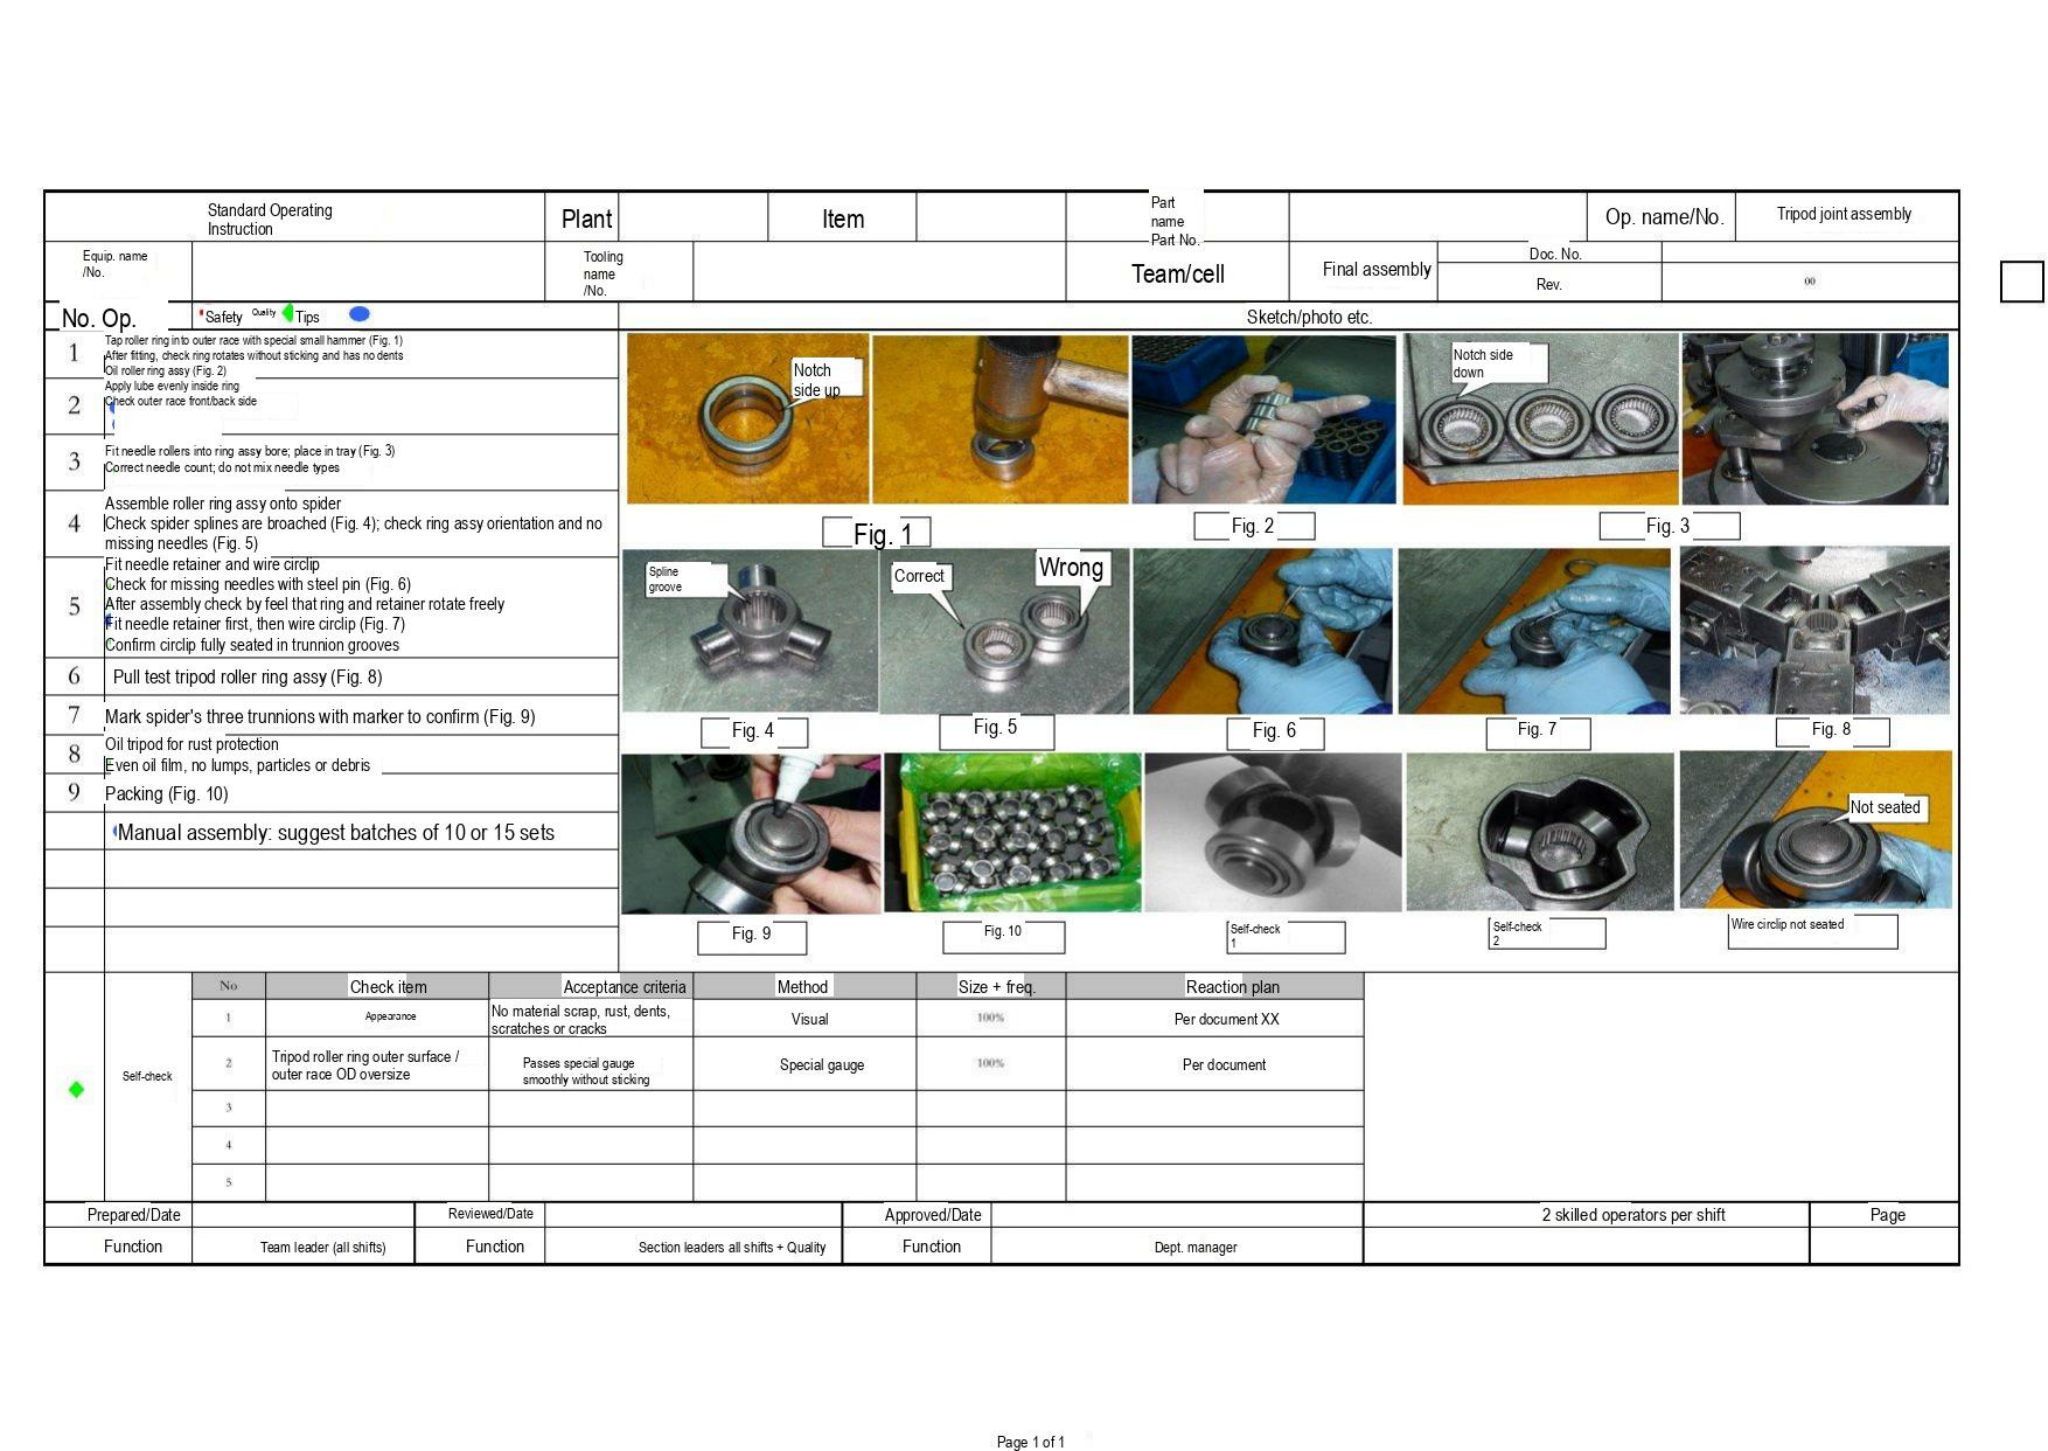Standard Operating Instruction | Plant | Item | Part name / Part No. | Op. name/No. | Tripod joint assembly

Equip. name /No. | Tooling name /No. | Team/cell | Final assembly | Doc. No. | Rev. | 00

No. Op. | Safety | Quality | Tips | Sketch/photo etc.

1 Tap roller ring into outer race with special small hammer (Fig. 1)
After fitting, check ring rotates without sticking and has no dents
Oil roller ring assy (Fig. 2)
Apply lube evenly inside ring

2 Check outer race front/back side

3 Fit needle rollers into ring assy bore; place in tray (Fig. 3)
Correct needle count; do not mix needle types

4 Assemble roller ring assy onto spider
Check spider splines are broached (Fig. 4); check ring assy orientation and no missing needles (Fig. 5)

5 Fit needle retainer and wire circlip
Check for missing needles with steel pin (Fig. 6)
After assembly check by feel that ring and retainer rotate freely
Fit needle retainer first, then wire circlip (Fig. 7)
Confirm circlip fully seated in trunnion grooves

6 Pull test tripod roller ring assy (Fig. 8)

7 Mark spider's three trunnions with marker to confirm (Fig. 9)

8 Oil tripod for rust protection
Even oil film, no lumps, particles or debris

9 Packing (Fig. 10)

Manual assembly: suggest batches of 10 or 15 sets

Notch side up
Fig. 1
Fig. 2
Notch side down
Fig. 3
Spline groove
Fig. 4
Correct
Wrong
Fig. 5
Fig. 6
Fig. 7
Fig. 8
Fig. 9
Fig. 10
Self-check 1
Self-check 2
Not seated
Wire circlip not seated

Self-check

| No | Check item | Acceptance criteria | Method | Size + freq. | Reaction plan |
|---|---|---|---|---|---|
| 1 | Appearance | No material scrap, rust, dents, scratches or cracks | Visual | 100% | Per document XX |
| 2 | Tripod roller ring outer surface / outer race OD oversize | Passes special gauge smoothly without sticking | Special gauge | 100% | Per document |
| 3 | | | | | |
| 4 | | | | | |
| 5 | | | | | |

| Prepared/Date | | Reviewed/Date | | Approved/Date | | 2 skilled operators per shift | Page |
|---|---|---|---|---|---|---|---|
| Function | Team leader (all shifts) | Function | Section leaders all shifts + Quality | Function | Dept. manager | | |

Page 1 of 1